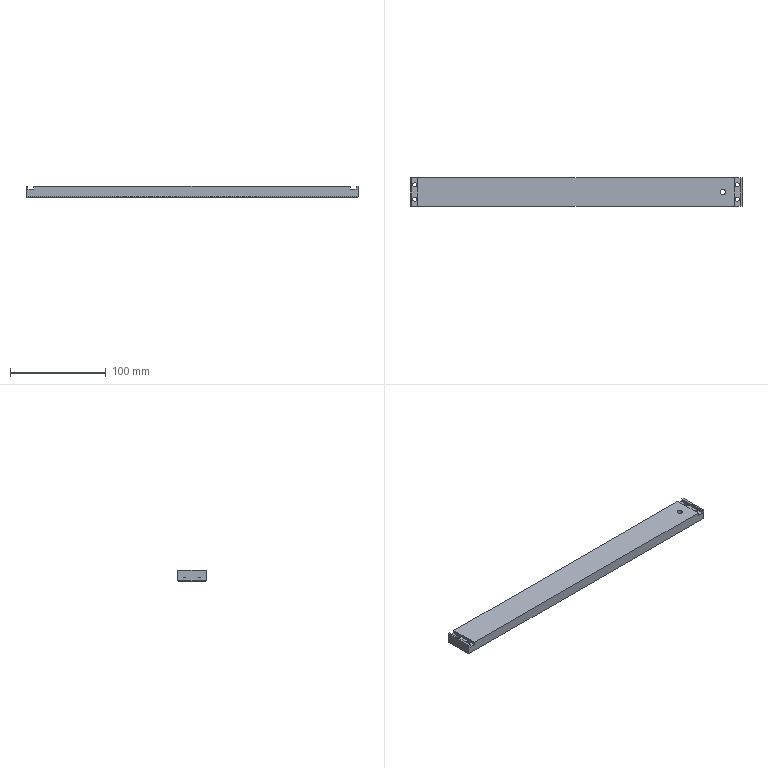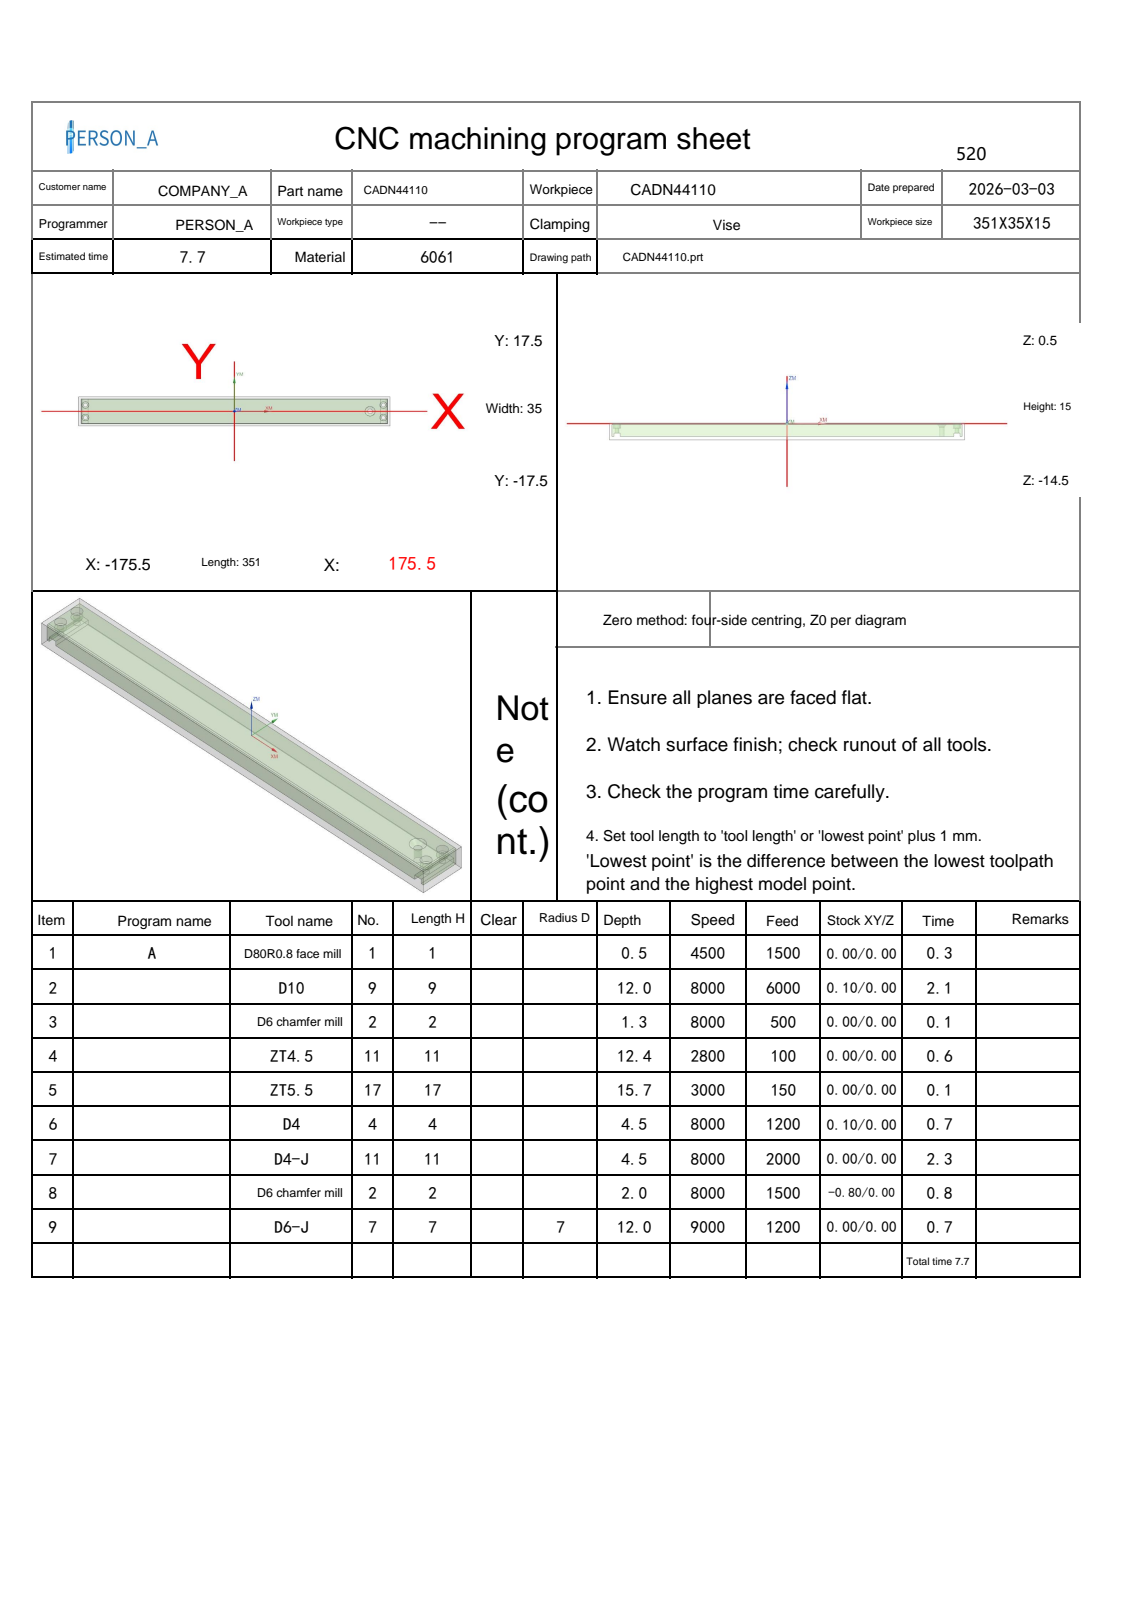NC program | NX | posted by the shop | part box 346 x 30 x 11.5 mm
Lines 28336 to 28539 of 28539:
N8 T02 M06
(D6 chamfer mill D=6. R=0. H=02 ce=-0.30 di=0.00)
G00 G90 G54 X171.212 Y8.247 M03 S8000
G43 H02 Z30.
M08
Z2.5
G01 X171.16 Y8.462 Z2.42 F500.
X171.024 Y8.828 Z2.278
X170.847 Y9.175 Z2.136
X170.629 Y9.499 Z1.994
X170.375 Y9.795 Z1.852
X170.088 Y10.059 Z1.71
X169.772 Y10.288 Z1.568
X169.528 Y10.428 Z1.465
X169.172 Y10.588 Z1.323
X168.8 Y10.705 Z1.181
X168.416 Y10.777 Z1.039
X168.027 Y10.803 Z.897
X167.638 Y10.783 Z.755
X167.253 Y10.717 Z.613
X166.879 Y10.607 Z.471
X166.52 Y10.453 Z.329
X166.182 Y10.258 Z.187
X165.87 Y10.024 Z.045
X165.587 Y9.756 Z-.097
X165.338 Y9.455 Z-.239
X165.126 Y9.128 Z-.381
X164.954 Y8.778 Z-.523
X164.825 Y8.41 Z-.665
X164.74 Y8.029 Z-.807
X164.7 Y7.641 Z-.949
Y7.5 Z-1.
G03 X168. Y4.2 I3.3 J0.0
X171.3 Y7.5 I0.0 J3.3
X168. Y10.8 I-3.3 J0.0
X164.7 Y7.5 I0.0 J-3.3
X164.738 Y7.002 I3.3 J0.0
G01 Z1.5
G00 Z30.
X171.212 Y-6.753
Z2.5
G01 X171.16 Y-6.538 Z2.42
X171.024 Y-6.172 Z2.278
X170.847 Y-5.825 Z2.136
X170.629 Y-5.501 Z1.994
X170.375 Y-5.205 Z1.852
X170.088 Y-4.941 Z1.71
X169.772 Y-4.712 Z1.568
X169.528 Y-4.572 Z1.465
X169.172 Y-4.412 Z1.323
X168.8 Y-4.295 Z1.181
X168.416 Y-4.223 Z1.039
X168.027 Y-4.197 Z.897
X167.638 Y-4.217 Z.755
X167.253 Y-4.283 Z.613
X166.879 Y-4.393 Z.471
X166.52 Y-4.547 Z.329
X166.182 Y-4.742 Z.187
X165.87 Y-4.976 Z.045
X165.587 Y-5.244 Z-.097
X165.338 Y-5.545 Z-.239
X165.126 Y-5.872 Z-.381
X164.954 Y-6.222 Z-.523
X164.825 Y-6.59 Z-.665
X164.74 Y-6.971 Z-.807
X164.7 Y-7.359 Z-.949
Y-7.5 Z-1.
G03 X168. Y-10.8 I3.3 J0.0
X171.3 Y-7.5 I0.0 J3.3
X168. Y-4.2 I-3.3 J0.0
X164.7 Y-7.5 I0.0 J-3.3
X164.738 Y-7.998 I3.3 J0.0
G01 Z1.5
G00 Z30.
X-164.788 Y-6.753
Z2.5
G01 X-164.84 Y-6.538 Z2.42
X-164.976 Y-6.172 Z2.278
X-165.153 Y-5.825 Z2.136
X-165.371 Y-5.501 Z1.994
X-165.625 Y-5.205 Z1.852
X-165.912 Y-4.941 Z1.71
X-166.228 Y-4.712 Z1.568
X-166.472 Y-4.572 Z1.465
X-166.828 Y-4.412 Z1.323
X-167.2 Y-4.295 Z1.181
X-167.584 Y-4.223 Z1.039
X-167.973 Y-4.197 Z.897
X-168.362 Y-4.217 Z.755
X-168.747 Y-4.283 Z.613
X-169.121 Y-4.393 Z.471
X-169.48 Y-4.547 Z.329
X-169.818 Y-4.742 Z.187
X-170.13 Y-4.976 Z.045
X-170.413 Y-5.244 Z-.097
X-170.662 Y-5.545 Z-.239
X-170.874 Y-5.872 Z-.381
X-171.046 Y-6.222 Z-.523
X-171.175 Y-6.59 Z-.665
X-171.26 Y-6.971 Z-.807
X-171.3 Y-7.359 Z-.949
Y-7.5 Z-1.
G03 X-168. Y-10.8 I3.3 J0.0
X-164.7 Y-7.5 I0.0 J3.3
X-168. Y-4.2 I-3.3 J0.0
X-171.3 Y-7.5 I0.0 J-3.3
X-171.262 Y-7.998 I3.3 J0.0
G01 Z1.5
G00 Z30.
X-164.788 Y8.247
Z2.5
G01 X-164.84 Y8.462 Z2.42
X-164.976 Y8.828 Z2.278
X-165.153 Y9.175 Z2.136
X-165.371 Y9.499 Z1.994
X-165.625 Y9.795 Z1.852
X-165.912 Y10.059 Z1.71
X-166.228 Y10.288 Z1.568
X-166.472 Y10.428 Z1.465
X-166.828 Y10.588 Z1.323
X-167.2 Y10.705 Z1.181
X-167.584 Y10.777 Z1.039
X-167.973 Y10.803 Z.897
X-168.362 Y10.783 Z.755
X-168.747 Y10.717 Z.613
X-169.121 Y10.607 Z.471
X-169.48 Y10.453 Z.329
X-169.818 Y10.258 Z.187
X-170.13 Y10.024 Z.045
X-170.413 Y9.756 Z-.097
X-170.662 Y9.455 Z-.239
X-170.874 Y9.128 Z-.381
X-171.046 Y8.778 Z-.523
X-171.175 Y8.41 Z-.665
X-171.26 Y8.029 Z-.807
X-171.3 Y7.641 Z-.949
Y7.5 Z-1.
G03 X-168. Y4.2 I3.3 J0.0
X-164.7 Y7.5 I0.0 J3.3
X-168. Y10.8 I-3.3 J0.0
X-171.3 Y7.5 I0.0 J-3.3
X-171.262 Y7.002 I3.3 J0.0
G01 Z1.5
G00 Z30.
G00 G90 X163.569 Y15.7 M03 S7000
Z30.
Z2.5
G01 X172.2 Z-.642 F1500.
X172.295 Z-.676
X172.533 Y15.666 Z-.764
X172.763 Y15.593 Z-.852
X172.979 Y15.486 Z-.939
X173.174 Y15.345 Z-1.027
X173.345 Y15.174 Z-1.115
X173.486 Y14.979 Z-1.202
X173.593 Y14.763 Z-1.29
X173.666 Y14.533 Z-1.378
X173.7 Y14.295 Z-1.465
Y14.2 Z-1.5
Y-14.2
G02 X172.2 Y-15.7 I-1.5 J0.0
G01 X-172.2
G02 X-173.7 Y-14.2 I0.0 J1.5
G01 Y14.2
G02 X-172.2 Y15.7 I1.5 J0.0
G01 X172.2
G02 X173.7 Y14.2 I0.0 J-1.5
G01 Y13.7
Z1.
G00 Z30.
G91 G28 Z0.0
M05
M09
G91 G28 Z0.0
M01
N9 T07 M06
(D6-J  D=6. R=0. H=07 ce=0.00 di=0.00)
G00 G90 G54 X-174.017 Y19.073 M03 S9000
G43 H07 Z30.
M08
Z-11.
G01 Z-11.5 F1200.
G41 D07
X-173.992 Y18.875
G03 X-173. Y18. I.992 J.125
G01 X173.
G02 X176. Y15. I0.0 J-3.
G01 Y-15.
G02 X173. Y-18. I-3. J0.0
G01 X-173.
G02 X-176. Y-15. I0.0 J3.
G01 Y15.
G02 X-173. Y18. I3. J0.0
G01 X-172.5
G03 X-171.5 Y19. I0.0 J1.
G01 G40 Y19.2
Z-11.
G00 Z30.
M05
M09
G91 G28 Z0.0
G91 G28 Y0.0
M30
%